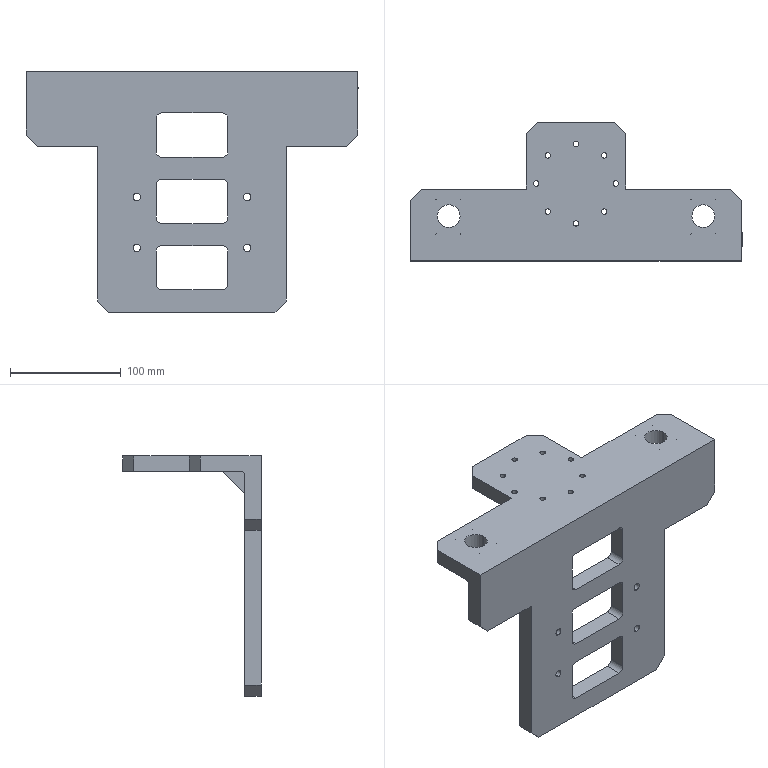Part | SolidWorks | features BaseBody 1 | 1 solid | 129 faces | box 300 x 125 x 217 mm | volume 835865 mm3 | cylinder 64 | plane 49 | cone 16 | commonest cylinder face diameters 4.2 x16 5 x16 10 x12 6.5 x8 11 x8 20.5 x4